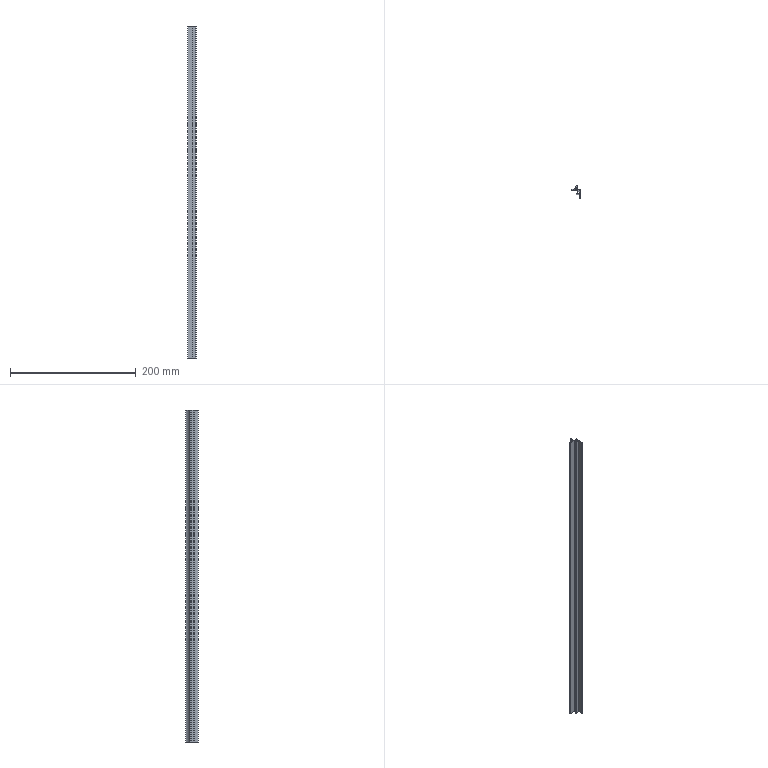Part | SolidWorks | features BaseBody 1, ICE 1, MoveFace 1 | 1 solid | 27 faces | box 14 x 20.3 x 528 mm | volume 26884 mm3 | plane 20 | cylinder 7 | commonest cylinder face diameters 0.387 x2 0.8 x2 0.4 x1 20 x1 22 x1
STEP:
#1=CARTESIAN_POINT('',(-5.304,-0.625,200.));
#2=VERTEX_POINT('',#1);
#3=CARTESIAN_POINT('',(-5.449,-0.8125,200.));
#4=VERTEX_POINT('',#3);
#5=CARTESIAN_POINT('',(-5.255,-0.8125,200.));
#6=DIRECTION('',(0.,0.,1.));
#7=DIRECTION('',(-1.,0.,0.));
#8=AXIS2_PLACEMENT_3D('',#5,#6,#7);
#9=CIRCLE('',#8,0.1937);
#10=EDGE_CURVE('',#2,#4,#9,.T.);
#11=ORIENTED_EDGE('',*,*,#10,.T.);
#12=CARTESIAN_POINT('',(-5.449,-0.8125,-328.));
#13=VERTEX_POINT('',#12);
#14=CARTESIAN_POINT('',(-5.449,-0.8125,230.));
#15=DIRECTION('',(0.,0.,-1.));
#16=VECTOR('',#15,1000.);
#17=LINE('',#14,#16);
#18=EDGE_CURVE('',#4,#13,#17,.T.);
#19=ORIENTED_EDGE('',*,*,#18,.T.);
#20=CARTESIAN_POINT('',(-5.304,-0.625,-328.));
#21=VERTEX_POINT('',#20);
#22=CARTESIAN_POINT('',(-5.255,-0.8125,-328.));
#23=DIRECTION('',(0.,0.,-1.));
#24=DIRECTION('',(1.,0.,0.));
#25=AXIS2_PLACEMENT_3D('',#22,#23,#24);
#26=CIRCLE('',#25,0.1937);
#27=EDGE_CURVE('',#13,#21,#26,.T.);
#28=ORIENTED_EDGE('',*,*,#27,.T.);
#29=CARTESIAN_POINT('',(-5.304,-0.625,230.));
#30=DIRECTION('',(0.,0.,-1.));
#31=VECTOR('',#30,1000.);
#32=LINE('',#29,#31);
#33=EDGE_CURVE('',#2,#21,#32,.T.);
#34=ORIENTED_EDGE('',*,*,#33,.F.);
#35=EDGE_LOOP('',(#11,#19,#28,#34));
#36=FACE_OUTER_BOUND('',#35,.T.);
#37=CARTESIAN_POINT('',(-5.255,-0.8125,230.));
#38=DIRECTION('',(0.,0.,-1.));
#39=DIRECTION('',(-1.,0.,0.));
#40=AXIS2_PLACEMENT_3D('',#37,#38,#39);
#41=CYLINDRICAL_SURFACE('',#40,0.1937);
#42=ADVANCED_FACE('',(#36),#41,.F.);
#43=CARTESIAN_POINT('',(5.,-1.,-328.));
#44=VERTEX_POINT('',#43);
#45=CARTESIAN_POINT('',(5.,-14.3,-328.));
#46=VERTEX_POINT('',#45);
#47=CARTESIAN_POINT('',(5.,29.623,-328.));
#48=DIRECTION('',(0.,-1.,0.));
#49=VECTOR('',#48,1000.);
#50=LINE('',#47,#49);
#51=EDGE_CURVE('',#44,#46,#50,.T.);
#52=ORIENTED_EDGE('',*,*,#51,.F.);
#53=CARTESIAN_POINT('',(5.,-1.,200.));
#54=VERTEX_POINT('',#53);
#55=CARTESIAN_POINT('',(5.,-1.,230.));
#56=DIRECTION('',(0.,0.,-1.));
#57=VECTOR('',#56,1000.);
#58=LINE('',#55,#57);
#59=EDGE_CURVE('',#54,#44,#58,.T.);
#60=ORIENTED_EDGE('',*,*,#59,.F.);
#61=CARTESIAN_POINT('',(5.,-14.3,200.));
#62=VERTEX_POINT('',#61);
#63=CARTESIAN_POINT('',(5.,-14.3,200.));
#64=DIRECTION('',(0.,1.,0.));
#65=VECTOR('',#64,1000.);
#66=LINE('',#63,#65);
#67=EDGE_CURVE('',#62,#54,#66,.T.);
#68=ORIENTED_EDGE('',*,*,#67,.F.);
#69=CARTESIAN_POINT('',(5.,-14.3,230.));
#70=DIRECTION('',(0.,0.,1.));
#71=VECTOR('',#70,1000.);
#72=LINE('',#69,#71);
#73=EDGE_CURVE('',#46,#62,#72,.T.);
#74=ORIENTED_EDGE('',*,*,#73,.F.);
#75=EDGE_LOOP('',(#52,#60,#68,#74));
#76=FACE_OUTER_BOUND('',#75,.T.);
#77=CARTESIAN_POINT('',(5.,-14.3,230.));
#78=DIRECTION('',(-1.,0.,0.));
#79=DIRECTION('',(0.,0.,1.));
#80=AXIS2_PLACEMENT_3D('',#77,#78,#79);
#81=PLANE('',#80);
#82=ADVANCED_FACE('',(#76),#81,.F.);
#83=CARTESIAN_POINT('',(-9.,-2.,-328.));
#84=VERTEX_POINT('',#83);
#85=CARTESIAN_POINT('',(-9.,-2.,200.));
#86=VERTEX_POINT('',#85);
#87=CARTESIAN_POINT('',(-9.,-2.,230.));
#88=DIRECTION('',(0.,0.,1.));
#89=VECTOR('',#88,1000.);
#90=LINE('',#87,#89);
#91=EDGE_CURVE('',#84,#86,#90,.T.);
#92=ORIENTED_EDGE('',*,*,#91,.F.);
#93=CARTESIAN_POINT('',(0.9,-2.,-328.));
#94=VERTEX_POINT('',#93);
#95=CARTESIAN_POINT('',(5.,-2.,-328.));
#96=DIRECTION('',(-1.,0.,0.));
#97=VECTOR('',#96,1000.);
#98=LINE('',#95,#97);
#99=EDGE_CURVE('',#94,#84,#98,.T.);
#100=ORIENTED_EDGE('',*,*,#99,.F.);
#101=CARTESIAN_POINT('',(0.9,-2.,200.));
#102=VERTEX_POINT('',#101);
#103=CARTESIAN_POINT('',(0.9,-2.,230.));
#104=DIRECTION('',(0.,0.,-1.));
#105=VECTOR('',#104,1000.);
#106=LINE('',#103,#105);
#107=EDGE_CURVE('',#102,#94,#106,.T.);
#108=ORIENTED_EDGE('',*,*,#107,.F.);
#109=CARTESIAN_POINT('',(5.,-2.,200.));
#110=DIRECTION('',(1.,0.,0.));
#111=VECTOR('',#110,1000.);
#112=LINE('',#109,#111);
#113=EDGE_CURVE('',#86,#102,#112,.T.);
#114=ORIENTED_EDGE('',*,*,#113,.F.);
#115=EDGE_LOOP('',(#92,#100,#108,#114));
#116=FACE_OUTER_BOUND('',#115,.T.);
#117=CARTESIAN_POINT('',(-9.,-2.,230.));
#118=DIRECTION('',(0.,1.,0.));
#119=DIRECTION('',(0.,0.,1.));
#120=AXIS2_PLACEMENT_3D('',#117,#118,#119);
#121=PLANE('',#120);
#122=ADVANCED_FACE('',(#116),#121,.F.);
#123=CARTESIAN_POINT('',(4.,-6.,200.));
#124=VERTEX_POINT('',#123);
#125=CARTESIAN_POINT('',(4.,-3.,200.));
#126=VERTEX_POINT('',#125);
#127=CARTESIAN_POINT('',(4.,29.623,200.));
#128=DIRECTION('',(0.,1.,0.));
#129=VECTOR('',#128,1000.);
#130=LINE('',#127,#129);
#131=EDGE_CURVE('',#124,#126,#130,.T.);
#132=ORIENTED_EDGE('',*,*,#131,.F.);
#133=CARTESIAN_POINT('',(1.,-6.,200.));
#134=VERTEX_POINT('',#133);
#135=CARTESIAN_POINT('',(5.,-6.,200.));
#136=DIRECTION('',(1.,0.,0.));
#137=VECTOR('',#136,1000.);
#138=LINE('',#135,#137);
#139=EDGE_CURVE('',#134,#124,#138,.T.);
#140=ORIENTED_EDGE('',*,*,#139,.F.);
#141=CARTESIAN_POINT('',(1.,-6.7,200.));
#142=VERTEX_POINT('',#141);
#143=CARTESIAN_POINT('',(1.,-6.,200.));
#144=DIRECTION('',(0.,-1.,0.));
#145=VECTOR('',#144,1000.);
#146=LINE('',#143,#145);
#147=EDGE_CURVE('',#134,#142,#146,.T.);
#148=ORIENTED_EDGE('',*,*,#147,.T.);
#149=CARTESIAN_POINT('',(-1.7,-6.7,200.));
#150=VERTEX_POINT('',#149);
#151=CARTESIAN_POINT('',(5.,-6.7,200.));
#152=DIRECTION('',(1.,0.,0.));
#153=VECTOR('',#152,1000.);
#154=LINE('',#151,#153);
#155=EDGE_CURVE('',#150,#142,#154,.T.);
#156=ORIENTED_EDGE('',*,*,#155,.F.);
#157=CARTESIAN_POINT('',(-1.7,-7.7,200.));
#158=VERTEX_POINT('',#157);
#159=CARTESIAN_POINT('',(-1.7,-6.7,200.));
#160=DIRECTION('',(0.,-1.,0.));
#161=VECTOR('',#160,1000.);
#162=LINE('',#159,#161);
#163=EDGE_CURVE('',#150,#158,#162,.T.);
#164=ORIENTED_EDGE('',*,*,#163,.T.);
#165=CARTESIAN_POINT('',(4.,-7.7,200.));
#166=VERTEX_POINT('',#165);
#167=CARTESIAN_POINT('',(5.,-7.7,200.));
#168=DIRECTION('',(-1.,0.,0.));
#169=VECTOR('',#168,1000.);
#170=LINE('',#167,#169);
#171=EDGE_CURVE('',#166,#158,#170,.T.);
#172=ORIENTED_EDGE('',*,*,#171,.F.);
#173=CARTESIAN_POINT('',(4.,-14.3,200.));
#174=VERTEX_POINT('',#173);
#175=CARTESIAN_POINT('',(4.,29.623,200.));
#176=DIRECTION('',(0.,1.,0.));
#177=VECTOR('',#176,1000.);
#178=LINE('',#175,#177);
#179=EDGE_CURVE('',#174,#166,#178,.T.);
#180=ORIENTED_EDGE('',*,*,#179,.F.);
#181=CARTESIAN_POINT('',(5.,-14.3,200.));
#182=DIRECTION('',(-1.,0.,0.));
#183=VECTOR('',#182,1000.);
#184=LINE('',#181,#183);
#185=EDGE_CURVE('',#62,#174,#184,.T.);
#186=ORIENTED_EDGE('',*,*,#185,.F.);
#187=ORIENTED_EDGE('',*,*,#67,.T.);
#188=CARTESIAN_POINT('',(-5.207,-1.,200.));
#189=VERTEX_POINT('',#188);
#190=CARTESIAN_POINT('',(5.,-1.,200.));
#191=DIRECTION('',(1.,0.,0.));
#192=VECTOR('',#191,1000.);
#193=LINE('',#190,#192);
#194=EDGE_CURVE('',#189,#54,#193,.T.);
#195=ORIENTED_EDGE('',*,*,#194,.F.);
#196=CARTESIAN_POINT('',(-5.255,-0.8125,200.));
#197=DIRECTION('',(0.,0.,1.));
#198=DIRECTION('',(-1.,0.,0.));
#199=AXIS2_PLACEMENT_3D('',#196,#197,#198);
#200=CIRCLE('',#199,0.1937);
#201=EDGE_CURVE('',#4,#189,#200,.T.);
#202=ORIENTED_EDGE('',*,*,#201,.F.);
#203=ORIENTED_EDGE('',*,*,#10,.F.);
#204=CARTESIAN_POINT('',(-1.368,3.063,200.));
#205=VERTEX_POINT('',#204);
#206=CARTESIAN_POINT('',(-10.628,9.,200.));
#207=DIRECTION('',(0.,0.,1.));
#208=DIRECTION('',(-1.,0.,0.));
#209=AXIS2_PLACEMENT_3D('',#206,#207,#208);
#210=CIRCLE('',#209,11.);
#211=EDGE_CURVE('',#2,#205,#210,.T.);
#212=ORIENTED_EDGE('',*,*,#211,.T.);
#213=CARTESIAN_POINT('',(-1.,2.955,200.));
#214=VERTEX_POINT('',#213);
#215=CARTESIAN_POINT('',(-1.2,2.955,200.));
#216=DIRECTION('',(0.,0.,1.));
#217=DIRECTION('',(-1.,0.,0.));
#218=AXIS2_PLACEMENT_3D('',#215,#216,#217);
#219=CIRCLE('',#218,0.2);
#220=EDGE_CURVE('',#214,#205,#219,.T.);
#221=ORIENTED_EDGE('',*,*,#220,.F.);
#222=CARTESIAN_POINT('',(-1.,1.5,200.));
#223=VERTEX_POINT('',#222);
#224=CARTESIAN_POINT('',(-1.,2.955,200.));
#225=DIRECTION('',(0.,1.,0.));
#226=VECTOR('',#225,1000.);
#227=LINE('',#224,#226);
#228=EDGE_CURVE('',#223,#214,#227,.T.);
#229=ORIENTED_EDGE('',*,*,#228,.F.);
#230=CARTESIAN_POINT('',(0.,1.5,200.));
#231=VERTEX_POINT('',#230);
#232=CARTESIAN_POINT('',(-1.,1.5,200.));
#233=DIRECTION('',(-1.,0.,0.));
#234=VECTOR('',#233,1000.);
#235=LINE('',#232,#234);
#236=EDGE_CURVE('',#231,#223,#235,.T.);
#237=ORIENTED_EDGE('',*,*,#236,.F.);
#238=CARTESIAN_POINT('',(0.,6.,200.));
#239=VERTEX_POINT('',#238);
#240=CARTESIAN_POINT('',(0.,1.5,200.));
#241=DIRECTION('',(0.,-1.,0.));
#242=VECTOR('',#241,1000.);
#243=LINE('',#240,#242);
#244=EDGE_CURVE('',#239,#231,#243,.T.);
#245=ORIENTED_EDGE('',*,*,#244,.F.);
#246=CARTESIAN_POINT('',(-0.8,6.,200.));
#247=VERTEX_POINT('',#246);
#248=CARTESIAN_POINT('',(0.,6.,200.));
#249=DIRECTION('',(1.,0.,0.));
#250=VECTOR('',#249,1000.);
#251=LINE('',#248,#250);
#252=EDGE_CURVE('',#247,#239,#251,.T.);
#253=ORIENTED_EDGE('',*,*,#252,.F.);
#254=CARTESIAN_POINT('',(-1.178,5.731,200.));
#255=VERTEX_POINT('',#254);
#256=CARTESIAN_POINT('',(-0.8,5.6,200.));
#257=DIRECTION('',(0.,0.,1.));
#258=DIRECTION('',(-1.,0.,0.));
#259=AXIS2_PLACEMENT_3D('',#256,#257,#258);
#260=CIRCLE('',#259,0.4);
#261=EDGE_CURVE('',#247,#255,#260,.T.);
#262=ORIENTED_EDGE('',*,*,#261,.T.);
#263=CARTESIAN_POINT('',(-8.678,-0.8077,200.));
#264=VERTEX_POINT('',#263);
#265=CARTESIAN_POINT('',(-10.628,9.,200.));
#266=DIRECTION('',(0.,0.,1.));
#267=DIRECTION('',(-1.,0.,0.));
#268=AXIS2_PLACEMENT_3D('',#265,#266,#267);
#269=CIRCLE('',#268,10.);
#270=EDGE_CURVE('',#264,#255,#269,.T.);
#271=ORIENTED_EDGE('',*,*,#270,.F.);
#272=CARTESIAN_POINT('',(-9.,-1.2,200.));
#273=VERTEX_POINT('',#272);
#274=CARTESIAN_POINT('',(-8.6,-1.2,200.));
#275=DIRECTION('',(0.,0.,1.));
#276=DIRECTION('',(-1.,0.,0.));
#277=AXIS2_PLACEMENT_3D('',#274,#275,#276);
#278=CIRCLE('',#277,0.4);
#279=EDGE_CURVE('',#264,#273,#278,.T.);
#280=ORIENTED_EDGE('',*,*,#279,.T.);
#281=CARTESIAN_POINT('',(-9.,8.,200.));
#282=DIRECTION('',(0.,-1.,0.));
#283=VECTOR('',#282,1000.);
#284=LINE('',#281,#283);
#285=EDGE_CURVE('',#273,#86,#284,.T.);
#286=ORIENTED_EDGE('',*,*,#285,.T.);
#287=ORIENTED_EDGE('',*,*,#113,.T.);
#288=CARTESIAN_POINT('',(0.9,-3.,200.));
#289=VERTEX_POINT('',#288);
#290=CARTESIAN_POINT('',(0.9,29.623,200.));
#291=DIRECTION('',(0.,1.,0.));
#292=VECTOR('',#291,1000.);
#293=LINE('',#290,#292);
#294=EDGE_CURVE('',#289,#102,#293,.T.);
#295=ORIENTED_EDGE('',*,*,#294,.F.);
#296=CARTESIAN_POINT('',(5.,-3.,200.));
#297=DIRECTION('',(-1.,0.,0.));
#298=VECTOR('',#297,1000.);
#299=LINE('',#296,#298);
#300=EDGE_CURVE('',#126,#289,#299,.T.);
#301=ORIENTED_EDGE('',*,*,#300,.F.);
#302=EDGE_LOOP('',(#132,#140,#148,#156,#164,#172,#180,#186,#187,#195,#202,#203,#212,#221,#229,#237,#245,#253,#262,#271,#280,#286,#287,#295,#301));
#303=FACE_OUTER_BOUND('',#302,.T.);
#304=CARTESIAN_POINT('',(5.,29.623,200.));
#305=DIRECTION('',(0.,0.,-1.));
#306=DIRECTION('',(-1.,0.,0.));
#307=AXIS2_PLACEMENT_3D('',#304,#305,#306);
#308=PLANE('',#307);
#309=ADVANCED_FACE('',(#303),#308,.F.);
#310=ORIENTED_EDGE('',*,*,#185,.T.);
#311=CARTESIAN_POINT('',(4.,-14.3,-328.));
#312=VERTEX_POINT('',#311);
#313=CARTESIAN_POINT('',(4.,-14.3,230.));
#314=DIRECTION('',(0.,0.,1.));
#315=VECTOR('',#314,1000.);
#316=LINE('',#313,#315);
#317=EDGE_CURVE('',#312,#174,#316,.T.);
#318=ORIENTED_EDGE('',*,*,#317,.F.);
#319=CARTESIAN_POINT('',(5.,-14.3,-328.));
#320=DIRECTION('',(-1.,0.,0.));
#321=VECTOR('',#320,1000.);
#322=LINE('',#319,#321);
#323=EDGE_CURVE('',#46,#312,#322,.T.);
#324=ORIENTED_EDGE('',*,*,#323,.F.);
#325=ORIENTED_EDGE('',*,*,#73,.T.);
#326=EDGE_LOOP('',(#310,#318,#324,#325));
#327=FACE_OUTER_BOUND('',#326,.T.);
#328=CARTESIAN_POINT('',(4.,-14.3,230.));
#329=DIRECTION('',(0.,1.,0.));
#330=DIRECTION('',(0.,0.,1.));
#331=AXIS2_PLACEMENT_3D('',#328,#329,#330);
#332=PLANE('',#331);
#333=ADVANCED_FACE('',(#327),#332,.F.);
#334=ORIENTED_EDGE('',*,*,#51,.T.);
#335=ORIENTED_EDGE('',*,*,#323,.T.);
#336=CARTESIAN_POINT('',(4.,-7.7,-328.));
#337=VERTEX_POINT('',#336);
#338=CARTESIAN_POINT('',(4.,-7.7,-328.));
#339=DIRECTION('',(0.,-1.,0.));
#340=VECTOR('',#339,1000.);
#341=LINE('',#338,#340);
#342=EDGE_CURVE('',#337,#312,#341,.T.);
#343=ORIENTED_EDGE('',*,*,#342,.F.);
#344=CARTESIAN_POINT('',(-1.7,-7.7,-328.));
#345=VERTEX_POINT('',#344);
#346=CARTESIAN_POINT('',(-1.7,-7.7,-328.));
#347=DIRECTION('',(1.,0.,0.));
#348=VECTOR('',#347,1000.);
#349=LINE('',#346,#348);
#350=EDGE_CURVE('',#345,#337,#349,.T.);
#351=ORIENTED_EDGE('',*,*,#350,.F.);
#352=CARTESIAN_POINT('',(-1.7,-6.7,-328.));
#353=VERTEX_POINT('',#352);
#354=CARTESIAN_POINT('',(-1.7,29.623,-328.));
#355=DIRECTION('',(0.,1.,0.));
#356=VECTOR('',#355,1000.);
#357=LINE('',#354,#356);
#358=EDGE_CURVE('',#345,#353,#357,.T.);
#359=ORIENTED_EDGE('',*,*,#358,.T.);
#360=CARTESIAN_POINT('',(1.,-6.7,-328.));
#361=VERTEX_POINT('',#360);
#362=CARTESIAN_POINT('',(1.,-6.7,-328.));
#363=DIRECTION('',(-1.,0.,0.));
#364=VECTOR('',#363,1000.);
#365=LINE('',#362,#364);
#366=EDGE_CURVE('',#361,#353,#365,.T.);
#367=ORIENTED_EDGE('',*,*,#366,.F.);
#368=CARTESIAN_POINT('',(1.,-6.,-328.));
#369=VERTEX_POINT('',#368);
#370=CARTESIAN_POINT('',(1.,29.623,-328.));
#371=DIRECTION('',(0.,1.,0.));
#372=VECTOR('',#371,1000.);
#373=LINE('',#370,#372);
#374=EDGE_CURVE('',#361,#369,#373,.T.);
#375=ORIENTED_EDGE('',*,*,#374,.T.);
#376=CARTESIAN_POINT('',(4.,-6.,-328.));
#377=VERTEX_POINT('',#376);
#378=CARTESIAN_POINT('',(4.,-6.,-328.));
#379=DIRECTION('',(-1.,0.,0.));
#380=VECTOR('',#379,1000.);
#381=LINE('',#378,#380);
#382=EDGE_CURVE('',#377,#369,#381,.T.);
#383=ORIENTED_EDGE('',*,*,#382,.F.);
#384=CARTESIAN_POINT('',(4.,-3.,-328.));
#385=VERTEX_POINT('',#384);
#386=CARTESIAN_POINT('',(4.,-3.,-328.));
#387=DIRECTION('',(0.,-1.,0.));
#388=VECTOR('',#387,1000.);
#389=LINE('',#386,#388);
#390=EDGE_CURVE('',#385,#377,#389,.T.);
#391=ORIENTED_EDGE('',*,*,#390,.F.);
#392=CARTESIAN_POINT('',(0.9,-3.,-328.));
#393=VERTEX_POINT('',#392);
#394=CARTESIAN_POINT('',(0.9,-3.,-328.));
#395=DIRECTION('',(1.,0.,0.));
#396=VECTOR('',#395,1000.);
#397=LINE('',#394,#396);
#398=EDGE_CURVE('',#393,#385,#397,.T.);
#399=ORIENTED_EDGE('',*,*,#398,.F.);
#400=CARTESIAN_POINT('',(0.9,-2.,-328.));
#401=DIRECTION('',(0.,-1.,0.));
#402=VECTOR('',#401,1000.);
#403=LINE('',#400,#402);
#404=EDGE_CURVE('',#94,#393,#403,.T.);
#405=ORIENTED_EDGE('',*,*,#404,.F.);
#406=ORIENTED_EDGE('',*,*,#99,.T.);
#407=CARTESIAN_POINT('',(-9.,-1.2,-328.));
#408=VERTEX_POINT('',#407);
#409=CARTESIAN_POINT('',(-9.,-1.2,-328.));
#410=DIRECTION('',(0.,-1.,0.));
#411=VECTOR('',#410,1000.);
#412=LINE('',#409,#411);
#413=EDGE_CURVE('',#408,#84,#412,.T.);
#414=ORIENTED_EDGE('',*,*,#413,.F.);
#415=CARTESIAN_POINT('',(-8.678,-0.8077,-328.));
#416=VERTEX_POINT('',#415);
#417=CARTESIAN_POINT('',(-8.6,-1.2,-328.));
#418=DIRECTION('',(0.,0.,-1.));
#419=DIRECTION('',(1.,0.,0.));
#420=AXIS2_PLACEMENT_3D('',#417,#418,#419);
#421=CIRCLE('',#420,0.4);
#422=EDGE_CURVE('',#408,#416,#421,.T.);
#423=ORIENTED_EDGE('',*,*,#422,.T.);
#424=CARTESIAN_POINT('',(-1.178,5.731,-328.));
#425=VERTEX_POINT('',#424);
#426=CARTESIAN_POINT('',(-10.628,9.,-328.));
#427=DIRECTION('',(0.,0.,-1.));
#428=DIRECTION('',(1.,0.,0.));
#429=AXIS2_PLACEMENT_3D('',#426,#427,#428);
#430=CIRCLE('',#429,10.);
#431=EDGE_CURVE('',#425,#416,#430,.T.);
#432=ORIENTED_EDGE('',*,*,#431,.F.);
#433=CARTESIAN_POINT('',(-0.8,6.,-328.));
#434=VERTEX_POINT('',#433);
#435=CARTESIAN_POINT('',(-0.8,5.6,-328.));
#436=DIRECTION('',(0.,0.,-1.));
#437=DIRECTION('',(1.,0.,0.));
#438=AXIS2_PLACEMENT_3D('',#435,#436,#437);
#439=CIRCLE('',#438,0.4);
#440=EDGE_CURVE('',#425,#434,#439,.T.);
#441=ORIENTED_EDGE('',*,*,#440,.T.);
#442=CARTESIAN_POINT('',(0.,6.,-328.));
#443=VERTEX_POINT('',#442);
#444=CARTESIAN_POINT('',(0.,6.,-328.));
#445=DIRECTION('',(-1.,0.,0.));
#446=VECTOR('',#445,1000.);
#447=LINE('',#444,#446);
#448=EDGE_CURVE('',#443,#434,#447,.T.);
#449=ORIENTED_EDGE('',*,*,#448,.F.);
#450=CARTESIAN_POINT('',(0.,1.5,-328.));
#451=VERTEX_POINT('',#450);
#452=CARTESIAN_POINT('',(0.,1.5,-328.));
#453=DIRECTION('',(0.,1.,0.));
#454=VECTOR('',#453,1000.);
#455=LINE('',#452,#454);
#456=EDGE_CURVE('',#451,#443,#455,.T.);
#457=ORIENTED_EDGE('',*,*,#456,.F.);
#458=CARTESIAN_POINT('',(-1.,1.5,-328.));
#459=VERTEX_POINT('',#458);
#460=CARTESIAN_POINT('',(-1.,1.5,-328.));
#461=DIRECTION('',(1.,0.,0.));
#462=VECTOR('',#461,1000.);
#463=LINE('',#460,#462);
#464=EDGE_CURVE('',#459,#451,#463,.T.);
#465=ORIENTED_EDGE('',*,*,#464,.F.);
#466=CARTESIAN_POINT('',(-1.,2.955,-328.));
#467=VERTEX_POINT('',#466);
#468=CARTESIAN_POINT('',(-1.,2.955,-328.));
#469=DIRECTION('',(0.,-1.,0.));
#470=VECTOR('',#469,1000.);
#471=LINE('',#468,#470);
#472=EDGE_CURVE('',#467,#459,#471,.T.);
#473=ORIENTED_EDGE('',*,*,#472,.F.);
#474=CARTESIAN_POINT('',(-1.368,3.063,-328.));
#475=VERTEX_POINT('',#474);
#476=CARTESIAN_POINT('',(-1.2,2.955,-328.));
#477=DIRECTION('',(0.,0.,-1.));
#478=DIRECTION('',(1.,0.,0.));
#479=AXIS2_PLACEMENT_3D('',#476,#477,#478);
#480=CIRCLE('',#479,0.2);
#481=EDGE_CURVE('',#475,#467,#480,.T.);
#482=ORIENTED_EDGE('',*,*,#481,.F.);
#483=CARTESIAN_POINT('',(-10.628,9.,-328.));
#484=DIRECTION('',(0.,0.,-1.));
#485=DIRECTION('',(1.,0.,0.));
#486=AXIS2_PLACEMENT_3D('',#483,#484,#485);
#487=CIRCLE('',#486,11.);
#488=EDGE_CURVE('',#475,#21,#487,.T.);
#489=ORIENTED_EDGE('',*,*,#488,.T.);
#490=ORIENTED_EDGE('',*,*,#27,.F.);
#491=CARTESIAN_POINT('',(-5.207,-1.,-328.));
#492=VERTEX_POINT('',#491);
#493=CARTESIAN_POINT('',(-5.255,-0.8125,-328.));
#494=DIRECTION('',(0.,0.,-1.));
#495=DIRECTION('',(1.,0.,0.));
#496=AXIS2_PLACEMENT_3D('',#493,#494,#495);
#497=CIRCLE('',#496,0.1937);
#498=EDGE_CURVE('',#492,#13,#497,.T.);
#499=ORIENTED_EDGE('',*,*,#498,.F.);
#500=CARTESIAN_POINT('',(5.,-1.,-328.));
#501=DIRECTION('',(-1.,0.,0.));
#502=VECTOR('',#501,1000.);
#503=LINE('',#500,#502);
#504=EDGE_CURVE('',#44,#492,#503,.T.);
#505=ORIENTED_EDGE('',*,*,#504,.F.);
#506=EDGE_LOOP('',(#334,#335,#343,#351,#359,#367,#375,#383,#391,#399,#405,#406,#414,#423,#432,#441,#449,#457,#465,#473,#482,#489,#490,#499,#505));
#507=FACE_OUTER_BOUND('',#506,.T.);
#508=CARTESIAN_POINT('',(5.,29.623,-328.));
#509=DIRECTION('',(0.,0.,1.));
#510=DIRECTION('',(1.,0.,0.));
#511=AXIS2_PLACEMENT_3D('',#508,#509,#510);
#512=PLANE('',#511);
#513=ADVANCED_FACE('',(#507),#512,.F.);
#514=ORIENTED_EDGE('',*,*,#59,.T.);
#515=ORIENTED_EDGE('',*,*,#504,.T.);
#516=CARTESIAN_POINT('',(-5.207,-1.,230.));
#517=DIRECTION('',(0.,0.,-1.));
#518=VECTOR('',#517,1000.);
#519=LINE('',#516,#518);
#520=EDGE_CURVE('',#189,#492,#519,.T.);
#521=ORIENTED_EDGE('',*,*,#520,.F.);
#522=ORIENTED_EDGE('',*,*,#194,.T.);
#523=EDGE_LOOP('',(#514,#515,#521,#522));
#524=FACE_OUTER_BOUND('',#523,.T.);
#525=CARTESIAN_POINT('',(5.,-1.,230.));
#526=DIRECTION('',(0.,-1.,0.));
#527=DIRECTION('',(0.,0.,-1.));
#528=AXIS2_PLACEMENT_3D('',#525,#526,#527);
#529=PLANE('',#528);
#530=ADVANCED_FACE('',(#524),#529,.F.);
#531=CARTESIAN_POINT('',(-9.,-1.2,230.));
#532=DIRECTION('',(0.,0.,1.));
#533=VECTOR('',#532,1000.);
#534=LINE('',#531,#533);
#535=EDGE_CURVE('',#408,#273,#534,.T.);
#536=ORIENTED_EDGE('',*,*,#535,.F.);
#537=ORIENTED_EDGE('',*,*,#413,.T.);
#538=ORIENTED_EDGE('',*,*,#91,.T.);
#539=ORIENTED_EDGE('',*,*,#285,.F.);
#540=EDGE_LOOP('',(#536,#537,#538,#539));
#541=FACE_OUTER_BOUND('',#540,.T.);
#542=CARTESIAN_POINT('',(-9.,-1.2,230.));
#543=DIRECTION('',(1.,0.,0.));
#544=DIRECTION('',(0.,0.,-1.));
#545=AXIS2_PLACEMENT_3D('',#542,#543,#544);
#546=PLANE('',#545);
#547=ADVANCED_FACE('',(#541),#546,.F.);
#548=ORIENTED_EDGE('',*,*,#294,.T.);
#549=ORIENTED_EDGE('',*,*,#107,.T.);
#550=ORIENTED_EDGE('',*,*,#404,.T.);
#551=CARTESIAN_POINT('',(0.9,-3.,230.));
#552=DIRECTION('',(0.,0.,-1.));
#553=VECTOR('',#552,1000.);
#554=LINE('',#551,#553);
#555=EDGE_CURVE('',#289,#393,#554,.T.);
#556=ORIENTED_EDGE('',*,*,#555,.F.);
#557=EDGE_LOOP('',(#548,#549,#550,#556));
#558=FACE_OUTER_BOUND('',#557,.T.);
#559=CARTESIAN_POINT('',(0.9,-2.,230.));
#560=DIRECTION('',(1.,0.,0.));
#561=DIRECTION('',(0.,0.,-1.));
#562=AXIS2_PLACEMENT_3D('',#559,#560,#561);
#563=PLANE('',#562);
#564=ADVANCED_FACE('',(#558),#563,.F.);
#565=ORIENTED_EDGE('',*,*,#300,.T.);
#566=ORIENTED_EDGE('',*,*,#555,.T.);
#567=ORIENTED_EDGE('',*,*,#398,.T.);
#568=CARTESIAN_POINT('',(4.,-3.,230.));
#569=DIRECTION('',(0.,0.,-1.));
#570=VECTOR('',#569,1000.);
#571=LINE('',#568,#570);
#572=EDGE_CURVE('',#126,#385,#571,.T.);
#573=ORIENTED_EDGE('',*,*,#572,.F.);
#574=EDGE_LOOP('',(#565,#566,#567,#573));
#575=FACE_OUTER_BOUND('',#574,.T.);
#576=CARTESIAN_POINT('',(0.9,-3.,230.));
#577=DIRECTION('',(0.,1.,0.));
#578=DIRECTION('',(0.,0.,1.));
#579=AXIS2_PLACEMENT_3D('',#576,#577,#578);
#580=PLANE('',#579);
#581=ADVANCED_FACE('',(#575),#580,.F.);
#582=ORIENTED_EDGE('',*,*,#131,.T.);
#583=ORIENTED_EDGE('',*,*,#572,.T.);
#584=ORIENTED_EDGE('',*,*,#390,.T.);
#585=CARTESIAN_POINT('',(4.,-6.,230.));
#586=DIRECTION('',(0.,0.,-1.));
#587=VECTOR('',#586,1000.);
#588=LINE('',#585,#587);
#589=EDGE_CURVE('',#124,#377,#588,.T.);
#590=ORIENTED_EDGE('',*,*,#589,.F.);
#591=EDGE_LOOP('',(#582,#583,#584,#590));
#592=FACE_OUTER_BOUND('',#591,.T.);
#593=CARTESIAN_POINT('',(4.,-3.,230.));
#594=DIRECTION('',(1.,0.,0.));
#595=DIRECTION('',(0.,0.,-1.));
#596=AXIS2_PLACEMENT_3D('',#593,#594,#595);
#597=PLANE('',#596);
#598=ADVANCED_FACE('',(#592),#597,.F.);
#599=ORIENTED_EDGE('',*,*,#139,.T.);
#600=ORIENTED_EDGE('',*,*,#589,.T.);
#601=ORIENTED_EDGE('',*,*,#382,.T.);
#602=CARTESIAN_POINT('',(1.,-6.,230.));
#603=DIRECTION('',(0.,0.,-1.));
#604=VECTOR('',#603,1000.);
#605=LINE('',#602,#604);
#606=EDGE_CURVE('',#134,#369,#605,.T.);
#607=ORIENTED_EDGE('',*,*,#606,.F.);
#608=EDGE_LOOP('',(#599,#600,#601,#607));
#609=FACE_OUTER_BOUND('',#608,.T.);
#610=CARTESIAN_POINT('',(4.,-6.,230.));
#611=DIRECTION('',(0.,-1.,0.));
#612=DIRECTION('',(0.,0.,-1.));
#613=AXIS2_PLACEMENT_3D('',#610,#611,#612);
#614=PLANE('',#613);
#615=ADVANCED_FACE('',(#609),#614,.F.);
#616=ORIENTED_EDGE('',*,*,#155,.T.);
#617=CARTESIAN_POINT('',(1.,-6.7,230.));
#618=DIRECTION('',(0.,0.,1.));
#619=VECTOR('',#618,1000.);
#620=LINE('',#617,#619);
#621=EDGE_CURVE('',#361,#142,#620,.T.);
#622=ORIENTED_EDGE('',*,*,#621,.F.);
#623=ORIENTED_EDGE('',*,*,#366,.T.);
#624=CARTESIAN_POINT('',(-1.7,-6.7,230.));
#625=DIRECTION('',(0.,0.,-1.));
#626=VECTOR('',#625,1000.);
#627=LINE('',#624,#626);
#628=EDGE_CURVE('',#150,#353,#627,.T.);
#629=ORIENTED_EDGE('',*,*,#628,.F.);
#630=EDGE_LOOP('',(#616,#622,#623,#629));
#631=FACE_OUTER_BOUND('',#630,.T.);
#632=CARTESIAN_POINT('',(1.,-6.7,230.));
#633=DIRECTION('',(0.,-1.,0.));
#634=DIRECTION('',(0.,0.,-1.));
#635=AXIS2_PLACEMENT_3D('',#632,#633,#634);
#636=PLANE('',#635);
#637=ADVANCED_FACE('',(#631),#636,.F.);
#638=ORIENTED_EDGE('',*,*,#171,.T.);
#639=CARTESIAN_POINT('',(-1.7,-7.7,230.));
#640=DIRECTION('',(0.,0.,1.));
#641=VECTOR('',#640,1000.);
#642=LINE('',#639,#641);
#643=EDGE_CURVE('',#345,#158,#642,.T.);
#644=ORIENTED_EDGE('',*,*,#643,.F.);
#645=ORIENTED_EDGE('',*,*,#350,.T.);
#646=CARTESIAN_POINT('',(4.,-7.7,230.));
#647=DIRECTION('',(0.,0.,-1.));
#648=VECTOR('',#647,1000.);
#649=LINE('',#646,#648);
#650=EDGE_CURVE('',#166,#337,#649,.T.);
#651=ORIENTED_EDGE('',*,*,#650,.F.);
#652=EDGE_LOOP('',(#638,#644,#645,#651));
#653=FACE_OUTER_BOUND('',#652,.T.);
#654=CARTESIAN_POINT('',(-1.7,-7.7,230.));
#655=DIRECTION('',(0.,1.,0.));
#656=DIRECTION('',(0.,0.,1.));
#657=AXIS2_PLACEMENT_3D('',#654,#655,#656);
#658=PLANE('',#657);
#659=ADVANCED_FACE('',(#653),#658,.F.);
#660=ORIENTED_EDGE('',*,*,#179,.T.);
#661=ORIENTED_EDGE('',*,*,#650,.T.);
#662=ORIENTED_EDGE('',*,*,#342,.T.);
#663=ORIENTED_EDGE('',*,*,#317,.T.);
#664=EDGE_LOOP('',(#660,#661,#662,#663));
#665=FACE_OUTER_BOUND('',#664,.T.);
#666=CARTESIAN_POINT('',(4.,-7.7,230.));
#667=DIRECTION('',(1.,0.,0.));
#668=DIRECTION('',(0.,0.,-1.));
#669=AXIS2_PLACEMENT_3D('',#666,#667,#668);
#670=PLANE('',#669);
#671=ADVANCED_FACE('',(#665),#670,.F.);
#672=ORIENTED_EDGE('',*,*,#18,.F.);
#673=ORIENTED_EDGE('',*,*,#201,.T.);
#674=ORIENTED_EDGE('',*,*,#520,.T.);
#675=ORIENTED_EDGE('',*,*,#498,.T.);
#676=EDGE_LOOP('',(#672,#673,#674,#675));
#677=FACE_OUTER_BOUND('',#676,.T.);
#678=CARTESIAN_POINT('',(-5.255,-0.8125,230.));
#679=DIRECTION('',(0.,0.,-1.));
#680=DIRECTION('',(-1.,0.,0.));
#681=AXIS2_PLACEMENT_3D('',#678,#679,#680);
#682=CYLINDRICAL_SURFACE('',#681,0.1937);
#683=ADVANCED_FACE('',(#677),#682,.F.);
#684=CARTESIAN_POINT('',(-1.,2.955,230.));
#685=DIRECTION('',(0.,0.,1.));
#686=VECTOR('',#685,1000.);
#687=LINE('',#684,#686);
#688=EDGE_CURVE('',#467,#214,#687,.T.);
#689=ORIENTED_EDGE('',*,*,#688,.F.);
#690=ORIENTED_EDGE('',*,*,#472,.T.);
#691=CARTESIAN_POINT('',(-1.,1.5,230.));
#692=DIRECTION('',(0.,0.,-1.));
#693=VECTOR('',#692,1000.);
#694=LINE('',#691,#693);
#695=EDGE_CURVE('',#223,#459,#694,.T.);
#696=ORIENTED_EDGE('',*,*,#695,.F.);
#697=ORIENTED_EDGE('',*,*,#228,.T.);
#698=EDGE_LOOP('',(#689,#690,#696,#697));
#699=FACE_OUTER_BOUND('',#698,.T.);
#700=CARTESIAN_POINT('',(-1.,2.955,230.));
#701=DIRECTION('',(1.,0.,0.));
#702=DIRECTION('',(0.,0.,-1.));
#703=AXIS2_PLACEMENT_3D('',#700,#701,#702);
#704=PLANE('',#703);
#705=ADVANCED_FACE('',(#699),#704,.F.);
#706=ORIENTED_EDGE('',*,*,#488,.F.);
#707=CARTESIAN_POINT('',(-1.368,3.063,230.));
#708=DIRECTION('',(0.,0.,1.));
#709=VECTOR('',#708,1000.);
#710=LINE('',#707,#709);
#711=EDGE_CURVE('',#475,#205,#710,.T.);
#712=ORIENTED_EDGE('',*,*,#711,.T.);
#713=ORIENTED_EDGE('',*,*,#211,.F.);
#714=ORIENTED_EDGE('',*,*,#33,.T.);
#715=EDGE_LOOP('',(#706,#712,#713,#714));
#716=FACE_OUTER_BOUND('',#715,.T.);
#717=CARTESIAN_POINT('',(-10.628,9.,230.));
#718=DIRECTION('',(0.,0.,-1.));
#719=DIRECTION('',(-1.,0.,0.));
#720=AXIS2_PLACEMENT_3D('',#717,#718,#719);
#721=CYLINDRICAL_SURFACE('',#720,11.);
#722=ADVANCED_FACE('',(#716),#721,.T.);
#723=CARTESIAN_POINT('',(-1.178,5.731,230.));
#724=DIRECTION('',(0.,0.,1.));
#725=VECTOR('',#724,1000.);
#726=LINE('',#723,#725);
#727=EDGE_CURVE('',#425,#255,#726,.T.);
#728=ORIENTED_EDGE('',*,*,#727,.F.);
#729=ORIENTED_EDGE('',*,*,#431,.T.);
#730=CARTESIAN_POINT('',(-8.678,-0.8077,230.));
#731=DIRECTION('',(0.,0.,-1.));
#732=VECTOR('',#731,1000.);
#733=LINE('',#730,#732);
#734=EDGE_CURVE('',#264,#416,#733,.T.);
#735=ORIENTED_EDGE('',*,*,#734,.F.);
#736=ORIENTED_EDGE('',*,*,#270,.T.);
#737=EDGE_LOOP('',(#728,#729,#735,#736));
#738=FACE_OUTER_BOUND('',#737,.T.);
#739=CARTESIAN_POINT('',(-10.628,9.,230.));
#740=DIRECTION('',(0.,0.,-1.));
#741=DIRECTION('',(-1.,0.,0.));
#742=AXIS2_PLACEMENT_3D('',#739,#740,#741);
#743=CYLINDRICAL_SURFACE('',#742,10.);
#744=ADVANCED_FACE('',(#738),#743,.F.);
#745=CARTESIAN_POINT('',(0.,1.5,230.));
#746=DIRECTION('',(0.,0.,1.));
#747=VECTOR('',#746,1000.);
#748=LINE('',#745,#747);
#749=EDGE_CURVE('',#451,#231,#748,.T.);
#750=ORIENTED_EDGE('',*,*,#749,.F.);
#751=ORIENTED_EDGE('',*,*,#456,.T.);
#752=CARTESIAN_POINT('',(0.,6.,230.));
#753=DIRECTION('',(0.,0.,-1.));
#754=VECTOR('',#753,1000.);
#755=LINE('',#752,#754);
#756=EDGE_CURVE('',#239,#443,#755,.T.);
#757=ORIENTED_EDGE('',*,*,#756,.F.);
#758=ORIENTED_EDGE('',*,*,#244,.T.);
#759=EDGE_LOOP('',(#750,#751,#757,#758));
#760=FACE_OUTER_BOUND('',#759,.T.);
#761=CARTESIAN_POINT('',(0.,1.5,230.));
#762=DIRECTION('',(-1.,0.,0.));
#763=DIRECTION('',(0.,0.,1.));
#764=AXIS2_PLACEMENT_3D('',#761,#762,#763);
#765=PLANE('',#764);
#766=ADVANCED_FACE('',(#760),#765,.F.);
#767=ORIENTED_EDGE('',*,*,#422,.F.);
#768=ORIENTED_EDGE('',*,*,#535,.T.);
#769=ORIENTED_EDGE('',*,*,#279,.F.);
#770=ORIENTED_EDGE('',*,*,#734,.T.);
#771=EDGE_LOOP('',(#767,#768,#769,#770));
#772=FACE_OUTER_BOUND('',#771,.T.);
#773=CARTESIAN_POINT('',(-8.6,-1.2,230.));
#774=DIRECTION('',(0.,0.,-1.));
#775=DIRECTION('',(-1.,0.,0.));
#776=AXIS2_PLACEMENT_3D('',#773,#774,#775);
#777=CYLINDRICAL_SURFACE('',#776,0.4);
#778=ADVANCED_FACE('',(#772),#777,.T.);
#779=ORIENTED_EDGE('',*,*,#147,.F.);
#780=ORIENTED_EDGE('',*,*,#606,.T.);
#781=ORIENTED_EDGE('',*,*,#374,.F.);
#782=ORIENTED_EDGE('',*,*,#621,.T.);
#783=EDGE_LOOP('',(#779,#780,#781,#782));
#784=FACE_OUTER_BOUND('',#783,.T.);
#785=CARTESIAN_POINT('',(1.,-6.,230.));
#786=DIRECTION('',(1.,0.,0.));
#787=DIRECTION('',(0.,0.,-1.));
#788=AXIS2_PLACEMENT_3D('',#785,#786,#787);
#789=PLANE('',#788);
#790=ADVANCED_FACE('',(#784),#789,.F.);
#791=ORIENTED_EDGE('',*,*,#163,.F.);
#792=ORIENTED_EDGE('',*,*,#628,.T.);
#793=ORIENTED_EDGE('',*,*,#358,.F.);
#794=ORIENTED_EDGE('',*,*,#643,.T.);
#795=EDGE_LOOP('',(#791,#792,#793,#794));
#796=FACE_OUTER_BOUND('',#795,.T.);
#797=CARTESIAN_POINT('',(-1.7,-6.7,230.));
#798=DIRECTION('',(1.,0.,0.));
#799=DIRECTION('',(0.,0.,-1.));
#800=AXIS2_PLACEMENT_3D('',#797,#798,#799);
#801=PLANE('',#800);
#802=ADVANCED_FACE('',(#796),#801,.F.);
#803=ORIENTED_EDGE('',*,*,#711,.F.);
#804=ORIENTED_EDGE('',*,*,#481,.T.);
#805=ORIENTED_EDGE('',*,*,#688,.T.);
#806=ORIENTED_EDGE('',*,*,#220,.T.);
#807=EDGE_LOOP('',(#803,#804,#805,#806));
#808=FACE_OUTER_BOUND('',#807,.T.);
#809=CARTESIAN_POINT('',(-1.2,2.955,230.));
#810=DIRECTION('',(0.,0.,-1.));
#811=DIRECTION('',(-1.,0.,0.));
#812=AXIS2_PLACEMENT_3D('',#809,#810,#811);
#813=CYLINDRICAL_SURFACE('',#812,0.2);
#814=ADVANCED_FACE('',(#808),#813,.F.);
#815=ORIENTED_EDGE('',*,*,#695,.T.);
#816=ORIENTED_EDGE('',*,*,#464,.T.);
#817=ORIENTED_EDGE('',*,*,#749,.T.);
#818=ORIENTED_EDGE('',*,*,#236,.T.);
#819=EDGE_LOOP('',(#815,#816,#817,#818));
#820=FACE_OUTER_BOUND('',#819,.T.);
#821=CARTESIAN_POINT('',(-1.,1.5,230.));
#822=DIRECTION('',(0.,1.,0.));
#823=DIRECTION('',(0.,0.,1.));
#824=AXIS2_PLACEMENT_3D('',#821,#822,#823);
#825=PLANE('',#824);
#826=ADVANCED_FACE('',(#820),#825,.F.);
#827=ORIENTED_EDGE('',*,*,#440,.F.);
#828=ORIENTED_EDGE('',*,*,#727,.T.);
#829=ORIENTED_EDGE('',*,*,#261,.F.);
#830=CARTESIAN_POINT('',(-0.8,6.,230.));
#831=DIRECTION('',(0.,0.,-1.));
#832=VECTOR('',#831,1000.);
#833=LINE('',#830,#832);
#834=EDGE_CURVE('',#247,#434,#833,.T.);
#835=ORIENTED_EDGE('',*,*,#834,.T.);
#836=EDGE_LOOP('',(#827,#828,#829,#835));
#837=FACE_OUTER_BOUND('',#836,.T.);
#838=CARTESIAN_POINT('',(-0.8,5.6,230.));
#839=DIRECTION('',(0.,0.,-1.));
#840=DIRECTION('',(-1.,0.,0.));
#841=AXIS2_PLACEMENT_3D('',#838,#839,#840);
#842=CYLINDRICAL_SURFACE('',#841,0.4);
#843=ADVANCED_FACE('',(#837),#842,.T.);
#844=ORIENTED_EDGE('',*,*,#756,.T.);
#845=ORIENTED_EDGE('',*,*,#448,.T.);
#846=ORIENTED_EDGE('',*,*,#834,.F.);
#847=ORIENTED_EDGE('',*,*,#252,.T.);
#848=EDGE_LOOP('',(#844,#845,#846,#847));
#849=FACE_OUTER_BOUND('',#848,.T.);
#850=CARTESIAN_POINT('',(0.,6.,230.));
#851=DIRECTION('',(0.,-1.,0.));
#852=DIRECTION('',(0.,0.,-1.));
#853=AXIS2_PLACEMENT_3D('',#850,#851,#852);
#854=PLANE('',#853);
#855=ADVANCED_FACE('',(#849),#854,.F.);
#856=CLOSED_SHELL('',(#42,#82,#122,#309,#333,#513,#530,#547,#564,#581,#598,#615,#637,#659,#671,#683,#705,#722,#744,#766,#778,#790,#802,#814,#826,#843,#855));
#857=MANIFOLD_SOLID_BREP('',#856);
#858=CARTESIAN_POINT('',(0.,0.,0.));
#859=DIRECTION('',(0.,0.,1.));
#860=DIRECTION('',(1.,0.,0.));
#861=AXIS2_PLACEMENT_3D('',#858,#859,#860);
#862=(LENGTH_UNIT()NAMED_UNIT(*)SI_UNIT(.MILLI.,.METRE.));
#863=UNCERTAINTY_MEASURE_WITH_UNIT(LENGTH_MEASURE(0.00001),#862,'','');
#864=(NAMED_UNIT(*)PLANE_ANGLE_UNIT()SI_UNIT($,.RADIAN.));
#865=(NAMED_UNIT(*)SI_UNIT($,.STERADIAN.)SOLID_ANGLE_UNIT());
#866=(GEOMETRIC_REPRESENTATION_CONTEXT(3)GLOBAL_UNCERTAINTY_ASSIGNED_CONTEXT((#863))GLOBAL_UNIT_ASSIGNED_CONTEXT((#862,#864,#865))REPRESENTATION_CONTEXT('',''));
#867=ADVANCED_BREP_SHAPE_REPRESENTATION('',(#857,#861),#866);